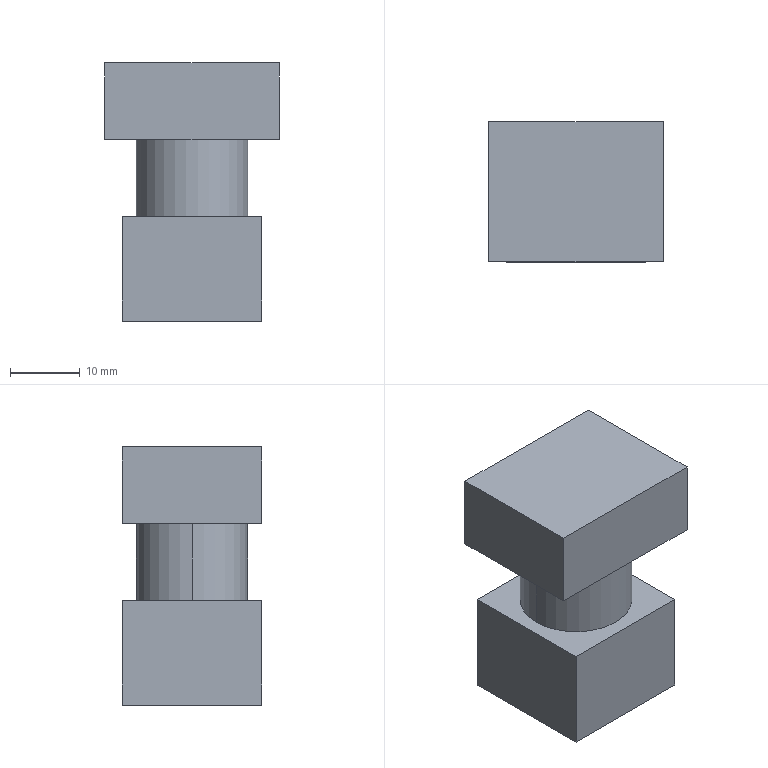Part | STEP file | Indicator light red | 1 solid | 14 faces | box 25 x 20 x 37 mm | volume 13712 mm3 | plane 12 | cylinder 2 | commonest cylinder face diameters 16 x2
STEP:
#1=CARTESIAN_POINT('',(0.,0.,0.));
#2=DIRECTION('',(0.,0.,1.));
#3=DIRECTION('',(1.,0.,0.));
#4=AXIS2_PLACEMENT_3D('',#1,#2,#3);
#5=CARTESIAN_POINT('',(8.,0.,-11.));
#6=VERTEX_POINT('',#5);
#7=CARTESIAN_POINT('',(-8.,0.,-11.));
#8=VERTEX_POINT('',#7);
#9=CARTESIAN_POINT('',(0.,0.,-11.));
#10=DIRECTION('',(0.,0.,1.));
#11=DIRECTION('',(1.,0.,0.));
#12=AXIS2_PLACEMENT_3D('',#9,#10,#11);
#13=CIRCLE('',#12,8.);
#14=CARTESIAN_POINT('',(0.,0.,-11.));
#15=DIRECTION('',(0.,0.,1.));
#16=DIRECTION('',(1.,0.,0.));
#17=AXIS2_PLACEMENT_3D('',#14,#15,#16);
#18=CYLINDRICAL_SURFACE('',#17,8.);
#19=CARTESIAN_POINT('',(0.,0.));
#20=DIRECTION('',(1.,0.));
#21=VECTOR('',#20,1.);
#22=LINE('',#19,#21);
#23=(GEOMETRIC_REPRESENTATION_CONTEXT(2)PARAMETRIC_REPRESENTATION_CONTEXT()REPRESENTATION_CONTEXT('',''));
#24=DEFINITIONAL_REPRESENTATION('',(#22),#23);
#25=PCURVE('',#18,#24);
#26=CARTESIAN_POINT('',(-10.,10.,-11.));
#27=DIRECTION('',(0.,0.,1.));
#28=DIRECTION('',(1.,0.,0.));
#29=AXIS2_PLACEMENT_3D('',#26,#27,#28);
#30=PLANE('',#29);
#31=CARTESIAN_POINT('',(10.,-10.));
#32=DIRECTION('',(1.,0.));
#33=AXIS2_PLACEMENT_2D('',#31,#32);
#34=CIRCLE('',#33,8.);
#35=(GEOMETRIC_REPRESENTATION_CONTEXT(2)PARAMETRIC_REPRESENTATION_CONTEXT()REPRESENTATION_CONTEXT('',''));
#36=DEFINITIONAL_REPRESENTATION('',(#34),#35);
#37=PCURVE('',#30,#36);
#38=SURFACE_CURVE('',#13,(#25,#37),.PCURVE_S1.);
#39=EDGE_CURVE('',#6,#8,#38,.T.);
#40=ORIENTED_EDGE('',*,*,#39,.T.);
#41=CARTESIAN_POINT('',(-8.,0.,0.));
#42=VERTEX_POINT('',#41);
#43=CARTESIAN_POINT('',(-8.,0.,-11.));
#44=DIRECTION('',(0.,0.,1.));
#45=VECTOR('',#44,1.);
#46=LINE('',#43,#45);
#47=CARTESIAN_POINT('',(3.142,0.));
#48=DIRECTION('',(0.,1.));
#49=VECTOR('',#48,1.);
#50=LINE('',#47,#49);
#51=(GEOMETRIC_REPRESENTATION_CONTEXT(2)PARAMETRIC_REPRESENTATION_CONTEXT()REPRESENTATION_CONTEXT('',''));
#52=DEFINITIONAL_REPRESENTATION('',(#50),#51);
#53=PCURVE('',#18,#52);
#54=CARTESIAN_POINT('',(0.,0.,-11.));
#55=DIRECTION('',(0.,0.,1.));
#56=DIRECTION('',(1.,0.,0.));
#57=AXIS2_PLACEMENT_3D('',#54,#55,#56);
#58=CYLINDRICAL_SURFACE('',#57,8.);
#59=CARTESIAN_POINT('',(3.142,0.));
#60=DIRECTION('',(0.,1.));
#61=VECTOR('',#60,1.);
#62=LINE('',#59,#61);
#63=(GEOMETRIC_REPRESENTATION_CONTEXT(2)PARAMETRIC_REPRESENTATION_CONTEXT()REPRESENTATION_CONTEXT('',''));
#64=DEFINITIONAL_REPRESENTATION('',(#62),#63);
#65=PCURVE('',#58,#64);
#66=SURFACE_CURVE('',#46,(#53,#65),.PCURVE_S1.);
#67=EDGE_CURVE('',#8,#42,#66,.T.);
#68=ORIENTED_EDGE('',*,*,#67,.T.);
#69=CARTESIAN_POINT('',(8.,0.,0.));
#70=VERTEX_POINT('',#69);
#71=CARTESIAN_POINT('',(0.,0.,0.));
#72=DIRECTION('',(0.,0.,-1.));
#73=DIRECTION('',(1.,0.,0.));
#74=AXIS2_PLACEMENT_3D('',#71,#72,#73);
#75=CIRCLE('',#74,8.);
#76=CARTESIAN_POINT('',(6.283,11.));
#77=DIRECTION('',(-1.,0.));
#78=VECTOR('',#77,1.);
#79=LINE('',#76,#78);
#80=(GEOMETRIC_REPRESENTATION_CONTEXT(2)PARAMETRIC_REPRESENTATION_CONTEXT()REPRESENTATION_CONTEXT('',''));
#81=DEFINITIONAL_REPRESENTATION('',(#79),#80);
#82=PCURVE('',#18,#81);
#83=CARTESIAN_POINT('',(12.5,-10.,0.));
#84=DIRECTION('',(0.,0.,1.));
#85=DIRECTION('',(1.,0.,0.));
#86=AXIS2_PLACEMENT_3D('',#83,#84,#85);
#87=PLANE('',#86);
#88=CARTESIAN_POINT('',(-4.5,10.));
#89=CARTESIAN_POINT('',(-4.5,-3.856));
#90=CARTESIAN_POINT('',(-16.5,3.072));
#91=CARTESIAN_POINT('',(-28.5,10.));
#92=CARTESIAN_POINT('',(-16.5,16.928));
#93=CARTESIAN_POINT('',(-4.5,23.856));
#94=CARTESIAN_POINT('',(-4.5,10.));
#95=(BOUNDED_CURVE()B_SPLINE_CURVE(2,(#88,#89,#90,#91,#92,#93,#94),.UNSPECIFIED.,.T.,.F.)B_SPLINE_CURVE_WITH_KNOTS((1,2,2,2,2,1),(-2.094,0.,2.094,4.189,6.283,8.378),.UNSPECIFIED.)CURVE()GEOMETRIC_REPRESENTATION_ITEM()RATIONAL_B_SPLINE_CURVE((1.,0.5,1.,0.5,1.,0.5,1.))REPRESENTATION_ITEM(''));
#96=(GEOMETRIC_REPRESENTATION_CONTEXT(2)PARAMETRIC_REPRESENTATION_CONTEXT()REPRESENTATION_CONTEXT('',''));
#97=DEFINITIONAL_REPRESENTATION('',(#95),#96);
#98=PCURVE('',#87,#97);
#99=SURFACE_CURVE('',#75,(#82,#98),.PCURVE_S1.);
#100=EDGE_CURVE('',#42,#70,#99,.T.);
#101=ORIENTED_EDGE('',*,*,#100,.T.);
#102=CARTESIAN_POINT('',(8.,0.,-11.));
#103=DIRECTION('',(0.,0.,1.));
#104=VECTOR('',#103,1.);
#105=LINE('',#102,#104);
#106=CARTESIAN_POINT('',(0.,0.));
#107=DIRECTION('',(0.,1.));
#108=VECTOR('',#107,1.);
#109=LINE('',#106,#108);
#110=(GEOMETRIC_REPRESENTATION_CONTEXT(2)PARAMETRIC_REPRESENTATION_CONTEXT()REPRESENTATION_CONTEXT('',''));
#111=DEFINITIONAL_REPRESENTATION('',(#109),#110);
#112=PCURVE('',#18,#111);
#113=CARTESIAN_POINT('',(6.283,0.));
#114=DIRECTION('',(0.,1.));
#115=VECTOR('',#114,1.);
#116=LINE('',#113,#115);
#117=(GEOMETRIC_REPRESENTATION_CONTEXT(2)PARAMETRIC_REPRESENTATION_CONTEXT()REPRESENTATION_CONTEXT('',''));
#118=DEFINITIONAL_REPRESENTATION('',(#116),#117);
#119=PCURVE('',#58,#118);
#120=SURFACE_CURVE('',#105,(#112,#119),.PCURVE_S1.);
#121=EDGE_CURVE('',#6,#70,#120,.T.);
#122=ORIENTED_EDGE('',*,*,#121,.F.);
#123=EDGE_LOOP('',(#40,#68,#101,#122));
#124=FACE_BOUND('',#123,.T.);
#125=ADVANCED_FACE('',(#124),#18,.T.);
#126=CARTESIAN_POINT('',(-12.5,10.,11.));
#127=VERTEX_POINT('',#126);
#128=CARTESIAN_POINT('',(-12.5,-10.,11.));
#129=VERTEX_POINT('',#128);
#130=CARTESIAN_POINT('',(-12.5,-10.,11.));
#131=DIRECTION('',(0.,-1.,0.));
#132=VECTOR('',#131,1.);
#133=LINE('',#130,#132);
#134=CARTESIAN_POINT('',(12.5,-10.,11.));
#135=DIRECTION('',(0.,0.,1.));
#136=DIRECTION('',(1.,0.,0.));
#137=AXIS2_PLACEMENT_3D('',#134,#135,#136);
#138=PLANE('',#137);
#139=CARTESIAN_POINT('',(-25.,0.));
#140=DIRECTION('',(0.,-1.));
#141=VECTOR('',#140,1.);
#142=LINE('',#139,#141);
#143=(GEOMETRIC_REPRESENTATION_CONTEXT(2)PARAMETRIC_REPRESENTATION_CONTEXT()REPRESENTATION_CONTEXT('',''));
#144=DEFINITIONAL_REPRESENTATION('',(#142),#143);
#145=PCURVE('',#138,#144);
#146=CARTESIAN_POINT('',(-12.5,10.,11.));
#147=DIRECTION('',(1.,0.,0.));
#148=DIRECTION('',(0.,1.,0.));
#149=AXIS2_PLACEMENT_3D('',#146,#147,#148);
#150=PLANE('',#149);
#151=CARTESIAN_POINT('',(-20.,0.));
#152=DIRECTION('',(-1.,0.));
#153=VECTOR('',#152,1.);
#154=LINE('',#151,#153);
#155=(GEOMETRIC_REPRESENTATION_CONTEXT(2)PARAMETRIC_REPRESENTATION_CONTEXT()REPRESENTATION_CONTEXT('',''));
#156=DEFINITIONAL_REPRESENTATION('',(#154),#155);
#157=PCURVE('',#150,#156);
#158=SURFACE_CURVE('',#133,(#145,#157),.PCURVE_S1.);
#159=EDGE_CURVE('',#127,#129,#158,.T.);
#160=ORIENTED_EDGE('',*,*,#159,.T.);
#161=CARTESIAN_POINT('',(12.5,-10.,11.));
#162=VERTEX_POINT('',#161);
#163=CARTESIAN_POINT('',(12.5,-10.,11.));
#164=DIRECTION('',(1.,0.,0.));
#165=VECTOR('',#164,1.);
#166=LINE('',#163,#165);
#167=CARTESIAN_POINT('',(0.,0.));
#168=DIRECTION('',(1.,0.));
#169=VECTOR('',#168,1.);
#170=LINE('',#167,#169);
#171=(GEOMETRIC_REPRESENTATION_CONTEXT(2)PARAMETRIC_REPRESENTATION_CONTEXT()REPRESENTATION_CONTEXT('',''));
#172=DEFINITIONAL_REPRESENTATION('',(#170),#171);
#173=PCURVE('',#138,#172);
#174=CARTESIAN_POINT('',(-12.5,-10.,11.));
#175=DIRECTION('',(0.,1.,0.));
#176=DIRECTION('',(0.,0.,1.));
#177=AXIS2_PLACEMENT_3D('',#174,#175,#176);
#178=PLANE('',#177);
#179=CARTESIAN_POINT('',(0.,25.));
#180=DIRECTION('',(0.,1.));
#181=VECTOR('',#180,1.);
#182=LINE('',#179,#181);
#183=(GEOMETRIC_REPRESENTATION_CONTEXT(2)PARAMETRIC_REPRESENTATION_CONTEXT()REPRESENTATION_CONTEXT('',''));
#184=DEFINITIONAL_REPRESENTATION('',(#182),#183);
#185=PCURVE('',#178,#184);
#186=SURFACE_CURVE('',#166,(#173,#185),.PCURVE_S1.);
#187=EDGE_CURVE('',#129,#162,#186,.T.);
#188=ORIENTED_EDGE('',*,*,#187,.T.);
#189=CARTESIAN_POINT('',(12.5,10.,11.));
#190=VERTEX_POINT('',#189);
#191=CARTESIAN_POINT('',(12.5,-10.,11.));
#192=DIRECTION('',(0.,1.,0.));
#193=VECTOR('',#192,1.);
#194=LINE('',#191,#193);
#195=CARTESIAN_POINT('',(0.,0.));
#196=DIRECTION('',(0.,1.));
#197=VECTOR('',#196,1.);
#198=LINE('',#195,#197);
#199=(GEOMETRIC_REPRESENTATION_CONTEXT(2)PARAMETRIC_REPRESENTATION_CONTEXT()REPRESENTATION_CONTEXT('',''));
#200=DEFINITIONAL_REPRESENTATION('',(#198),#199);
#201=PCURVE('',#138,#200);
#202=CARTESIAN_POINT('',(12.5,10.,11.));
#203=DIRECTION('',(-1.,0.,0.));
#204=DIRECTION('',(0.,-1.,0.));
#205=AXIS2_PLACEMENT_3D('',#202,#203,#204);
#206=PLANE('',#205);
#207=CARTESIAN_POINT('',(20.,0.));
#208=DIRECTION('',(-1.,0.));
#209=VECTOR('',#208,1.);
#210=LINE('',#207,#209);
#211=(GEOMETRIC_REPRESENTATION_CONTEXT(2)PARAMETRIC_REPRESENTATION_CONTEXT()REPRESENTATION_CONTEXT('',''));
#212=DEFINITIONAL_REPRESENTATION('',(#210),#211);
#213=PCURVE('',#206,#212);
#214=SURFACE_CURVE('',#194,(#201,#213),.PCURVE_S1.);
#215=EDGE_CURVE('',#162,#190,#214,.T.);
#216=ORIENTED_EDGE('',*,*,#215,.T.);
#217=CARTESIAN_POINT('',(12.5,10.,11.));
#218=DIRECTION('',(-1.,0.,0.));
#219=VECTOR('',#218,1.);
#220=LINE('',#217,#219);
#221=CARTESIAN_POINT('',(0.,20.));
#222=DIRECTION('',(-1.,0.));
#223=VECTOR('',#222,1.);
#224=LINE('',#221,#223);
#225=(GEOMETRIC_REPRESENTATION_CONTEXT(2)PARAMETRIC_REPRESENTATION_CONTEXT()REPRESENTATION_CONTEXT('',''));
#226=DEFINITIONAL_REPRESENTATION('',(#224),#225);
#227=PCURVE('',#138,#226);
#228=CARTESIAN_POINT('',(-12.5,10.,11.));
#229=DIRECTION('',(0.,-1.,0.));
#230=DIRECTION('',(0.,0.,-1.));
#231=AXIS2_PLACEMENT_3D('',#228,#229,#230);
#232=PLANE('',#231);
#233=CARTESIAN_POINT('',(0.,25.));
#234=DIRECTION('',(0.,-1.));
#235=VECTOR('',#234,1.);
#236=LINE('',#233,#235);
#237=(GEOMETRIC_REPRESENTATION_CONTEXT(2)PARAMETRIC_REPRESENTATION_CONTEXT()REPRESENTATION_CONTEXT('',''));
#238=DEFINITIONAL_REPRESENTATION('',(#236),#237);
#239=PCURVE('',#232,#238);
#240=SURFACE_CURVE('',#220,(#227,#239),.PCURVE_S1.);
#241=EDGE_CURVE('',#190,#127,#240,.T.);
#242=ORIENTED_EDGE('',*,*,#241,.T.);
#243=EDGE_LOOP('',(#160,#188,#216,#242));
#244=FACE_BOUND('',#243,.T.);
#245=ADVANCED_FACE('',(#244),#138,.T.);
#246=CARTESIAN_POINT('',(12.5,-10.,0.));
#247=VERTEX_POINT('',#246);
#248=CARTESIAN_POINT('',(12.5,-10.,11.));
#249=DIRECTION('',(0.,0.,-1.));
#250=VECTOR('',#249,1.);
#251=LINE('',#248,#250);
#252=CARTESIAN_POINT('',(0.,25.));
#253=DIRECTION('',(-1.,0.));
#254=VECTOR('',#253,1.);
#255=LINE('',#252,#254);
#256=(GEOMETRIC_REPRESENTATION_CONTEXT(2)PARAMETRIC_REPRESENTATION_CONTEXT()REPRESENTATION_CONTEXT('',''));
#257=DEFINITIONAL_REPRESENTATION('',(#255),#256);
#258=PCURVE('',#178,#257);
#259=CARTESIAN_POINT('',(20.,0.));
#260=DIRECTION('',(0.,-1.));
#261=VECTOR('',#260,1.);
#262=LINE('',#259,#261);
#263=(GEOMETRIC_REPRESENTATION_CONTEXT(2)PARAMETRIC_REPRESENTATION_CONTEXT()REPRESENTATION_CONTEXT('',''));
#264=DEFINITIONAL_REPRESENTATION('',(#262),#263);
#265=PCURVE('',#206,#264);
#266=SURFACE_CURVE('',#251,(#258,#265),.PCURVE_S1.);
#267=EDGE_CURVE('',#162,#247,#266,.T.);
#268=ORIENTED_EDGE('',*,*,#267,.F.);
#269=ORIENTED_EDGE('',*,*,#187,.F.);
#270=CARTESIAN_POINT('',(-12.5,-10.,0.));
#271=VERTEX_POINT('',#270);
#272=CARTESIAN_POINT('',(-12.5,-10.,11.));
#273=DIRECTION('',(0.,0.,1.));
#274=VECTOR('',#273,1.);
#275=LINE('',#272,#274);
#276=CARTESIAN_POINT('',(0.,0.));
#277=DIRECTION('',(1.,0.));
#278=VECTOR('',#277,1.);
#279=LINE('',#276,#278);
#280=(GEOMETRIC_REPRESENTATION_CONTEXT(2)PARAMETRIC_REPRESENTATION_CONTEXT()REPRESENTATION_CONTEXT('',''));
#281=DEFINITIONAL_REPRESENTATION('',(#279),#280);
#282=PCURVE('',#178,#281);
#283=CARTESIAN_POINT('',(-20.,0.));
#284=DIRECTION('',(0.,1.));
#285=VECTOR('',#284,1.);
#286=LINE('',#283,#285);
#287=(GEOMETRIC_REPRESENTATION_CONTEXT(2)PARAMETRIC_REPRESENTATION_CONTEXT()REPRESENTATION_CONTEXT('',''));
#288=DEFINITIONAL_REPRESENTATION('',(#286),#287);
#289=PCURVE('',#150,#288);
#290=SURFACE_CURVE('',#275,(#282,#289),.PCURVE_S1.);
#291=EDGE_CURVE('',#271,#129,#290,.T.);
#292=ORIENTED_EDGE('',*,*,#291,.F.);
#293=CARTESIAN_POINT('',(-12.5,-10.,0.));
#294=DIRECTION('',(-1.,0.,0.));
#295=VECTOR('',#294,1.);
#296=LINE('',#293,#295);
#297=CARTESIAN_POINT('',(-11.,0.));
#298=DIRECTION('',(0.,-1.));
#299=VECTOR('',#298,1.);
#300=LINE('',#297,#299);
#301=(GEOMETRIC_REPRESENTATION_CONTEXT(2)PARAMETRIC_REPRESENTATION_CONTEXT()REPRESENTATION_CONTEXT('',''));
#302=DEFINITIONAL_REPRESENTATION('',(#300),#301);
#303=PCURVE('',#178,#302);
#304=CARTESIAN_POINT('',(-25.,0.));
#305=DIRECTION('',(-1.,0.));
#306=VECTOR('',#305,1.);
#307=LINE('',#304,#306);
#308=(GEOMETRIC_REPRESENTATION_CONTEXT(2)PARAMETRIC_REPRESENTATION_CONTEXT()REPRESENTATION_CONTEXT('',''));
#309=DEFINITIONAL_REPRESENTATION('',(#307),#308);
#310=PCURVE('',#87,#309);
#311=SURFACE_CURVE('',#296,(#303,#310),.PCURVE_S1.);
#312=EDGE_CURVE('',#247,#271,#311,.T.);
#313=ORIENTED_EDGE('',*,*,#312,.F.);
#314=EDGE_LOOP('',(#268,#269,#292,#313));
#315=FACE_BOUND('',#314,.T.);
#316=ADVANCED_FACE('',(#315),#178,.F.);
#317=ORIENTED_EDGE('',*,*,#291,.T.);
#318=ORIENTED_EDGE('',*,*,#159,.F.);
#319=CARTESIAN_POINT('',(-12.5,10.,0.));
#320=VERTEX_POINT('',#319);
#321=CARTESIAN_POINT('',(-12.5,10.,11.));
#322=DIRECTION('',(0.,0.,1.));
#323=VECTOR('',#322,1.);
#324=LINE('',#321,#323);
#325=CARTESIAN_POINT('',(0.,0.));
#326=DIRECTION('',(0.,1.));
#327=VECTOR('',#326,1.);
#328=LINE('',#325,#327);
#329=(GEOMETRIC_REPRESENTATION_CONTEXT(2)PARAMETRIC_REPRESENTATION_CONTEXT()REPRESENTATION_CONTEXT('',''));
#330=DEFINITIONAL_REPRESENTATION('',(#328),#329);
#331=PCURVE('',#150,#330);
#332=CARTESIAN_POINT('',(0.,0.));
#333=DIRECTION('',(-1.,0.));
#334=VECTOR('',#333,1.);
#335=LINE('',#332,#334);
#336=(GEOMETRIC_REPRESENTATION_CONTEXT(2)PARAMETRIC_REPRESENTATION_CONTEXT()REPRESENTATION_CONTEXT('',''));
#337=DEFINITIONAL_REPRESENTATION('',(#335),#336);
#338=PCURVE('',#232,#337);
#339=SURFACE_CURVE('',#324,(#331,#338),.PCURVE_S1.);
#340=EDGE_CURVE('',#320,#127,#339,.T.);
#341=ORIENTED_EDGE('',*,*,#340,.F.);
#342=CARTESIAN_POINT('',(-12.5,10.,0.));
#343=DIRECTION('',(0.,1.,0.));
#344=VECTOR('',#343,1.);
#345=LINE('',#342,#344);
#346=CARTESIAN_POINT('',(0.,-11.));
#347=DIRECTION('',(1.,0.));
#348=VECTOR('',#347,1.);
#349=LINE('',#346,#348);
#350=(GEOMETRIC_REPRESENTATION_CONTEXT(2)PARAMETRIC_REPRESENTATION_CONTEXT()REPRESENTATION_CONTEXT('',''));
#351=DEFINITIONAL_REPRESENTATION('',(#349),#350);
#352=PCURVE('',#150,#351);
#353=CARTESIAN_POINT('',(-25.,20.));
#354=DIRECTION('',(0.,1.));
#355=VECTOR('',#354,1.);
#356=LINE('',#353,#355);
#357=(GEOMETRIC_REPRESENTATION_CONTEXT(2)PARAMETRIC_REPRESENTATION_CONTEXT()REPRESENTATION_CONTEXT('',''));
#358=DEFINITIONAL_REPRESENTATION('',(#356),#357);
#359=PCURVE('',#87,#358);
#360=SURFACE_CURVE('',#345,(#352,#359),.PCURVE_S1.);
#361=EDGE_CURVE('',#271,#320,#360,.T.);
#362=ORIENTED_EDGE('',*,*,#361,.F.);
#363=EDGE_LOOP('',(#317,#318,#341,#362));
#364=FACE_BOUND('',#363,.T.);
#365=ADVANCED_FACE('',(#364),#150,.F.);
#366=ORIENTED_EDGE('',*,*,#340,.T.);
#367=ORIENTED_EDGE('',*,*,#241,.F.);
#368=CARTESIAN_POINT('',(12.5,10.,0.));
#369=VERTEX_POINT('',#368);
#370=CARTESIAN_POINT('',(12.5,10.,11.));
#371=DIRECTION('',(0.,0.,1.));
#372=VECTOR('',#371,1.);
#373=LINE('',#370,#372);
#374=CARTESIAN_POINT('',(0.,25.));
#375=DIRECTION('',(-1.,0.));
#376=VECTOR('',#375,1.);
#377=LINE('',#374,#376);
#378=(GEOMETRIC_REPRESENTATION_CONTEXT(2)PARAMETRIC_REPRESENTATION_CONTEXT()REPRESENTATION_CONTEXT('',''));
#379=DEFINITIONAL_REPRESENTATION('',(#377),#378);
#380=PCURVE('',#232,#379);
#381=CARTESIAN_POINT('',(0.,0.));
#382=DIRECTION('',(0.,1.));
#383=VECTOR('',#382,1.);
#384=LINE('',#381,#383);
#385=(GEOMETRIC_REPRESENTATION_CONTEXT(2)PARAMETRIC_REPRESENTATION_CONTEXT()REPRESENTATION_CONTEXT('',''));
#386=DEFINITIONAL_REPRESENTATION('',(#384),#385);
#387=PCURVE('',#206,#386);
#388=SURFACE_CURVE('',#373,(#380,#387),.PCURVE_S1.);
#389=EDGE_CURVE('',#369,#190,#388,.T.);
#390=ORIENTED_EDGE('',*,*,#389,.F.);
#391=CARTESIAN_POINT('',(-12.5,10.,0.));
#392=DIRECTION('',(1.,0.,0.));
#393=VECTOR('',#392,1.);
#394=LINE('',#391,#393);
#395=CARTESIAN_POINT('',(11.,0.));
#396=DIRECTION('',(0.,1.));
#397=VECTOR('',#396,1.);
#398=LINE('',#395,#397);
#399=(GEOMETRIC_REPRESENTATION_CONTEXT(2)PARAMETRIC_REPRESENTATION_CONTEXT()REPRESENTATION_CONTEXT('',''));
#400=DEFINITIONAL_REPRESENTATION('',(#398),#399);
#401=PCURVE('',#232,#400);
#402=CARTESIAN_POINT('',(-25.,20.));
#403=DIRECTION('',(1.,0.));
#404=VECTOR('',#403,1.);
#405=LINE('',#402,#404);
#406=(GEOMETRIC_REPRESENTATION_CONTEXT(2)PARAMETRIC_REPRESENTATION_CONTEXT()REPRESENTATION_CONTEXT('',''));
#407=DEFINITIONAL_REPRESENTATION('',(#405),#406);
#408=PCURVE('',#87,#407);
#409=SURFACE_CURVE('',#394,(#401,#408),.PCURVE_S1.);
#410=EDGE_CURVE('',#320,#369,#409,.T.);
#411=ORIENTED_EDGE('',*,*,#410,.F.);
#412=EDGE_LOOP('',(#366,#367,#390,#411));
#413=FACE_BOUND('',#412,.T.);
#414=ADVANCED_FACE('',(#413),#232,.F.);
#415=ORIENTED_EDGE('',*,*,#389,.T.);
#416=ORIENTED_EDGE('',*,*,#215,.F.);
#417=ORIENTED_EDGE('',*,*,#267,.T.);
#418=CARTESIAN_POINT('',(12.5,10.,0.));
#419=DIRECTION('',(0.,-1.,0.));
#420=VECTOR('',#419,1.);
#421=LINE('',#418,#420);
#422=CARTESIAN_POINT('',(0.,-11.));
#423=DIRECTION('',(1.,0.));
#424=VECTOR('',#423,1.);
#425=LINE('',#422,#424);
#426=(GEOMETRIC_REPRESENTATION_CONTEXT(2)PARAMETRIC_REPRESENTATION_CONTEXT()REPRESENTATION_CONTEXT('',''));
#427=DEFINITIONAL_REPRESENTATION('',(#425),#426);
#428=PCURVE('',#206,#427);
#429=CARTESIAN_POINT('',(0.,20.));
#430=DIRECTION('',(0.,-1.));
#431=VECTOR('',#430,1.);
#432=LINE('',#429,#431);
#433=(GEOMETRIC_REPRESENTATION_CONTEXT(2)PARAMETRIC_REPRESENTATION_CONTEXT()REPRESENTATION_CONTEXT('',''));
#434=DEFINITIONAL_REPRESENTATION('',(#432),#433);
#435=PCURVE('',#87,#434);
#436=SURFACE_CURVE('',#421,(#428,#435),.PCURVE_S1.);
#437=EDGE_CURVE('',#369,#247,#436,.T.);
#438=ORIENTED_EDGE('',*,*,#437,.F.);
#439=EDGE_LOOP('',(#415,#416,#417,#438));
#440=FACE_BOUND('',#439,.T.);
#441=ADVANCED_FACE('',(#440),#206,.F.);
#442=CARTESIAN_POINT('',(0.,0.,0.));
#443=DIRECTION('',(0.,0.,-1.));
#444=DIRECTION('',(1.,0.,0.));
#445=AXIS2_PLACEMENT_3D('',#442,#443,#444);
#446=CIRCLE('',#445,8.);
#447=CARTESIAN_POINT('',(-4.5,10.));
#448=CARTESIAN_POINT('',(-4.5,-3.856));
#449=CARTESIAN_POINT('',(-16.5,3.072));
#450=CARTESIAN_POINT('',(-28.5,10.));
#451=CARTESIAN_POINT('',(-16.5,16.928));
#452=CARTESIAN_POINT('',(-4.5,23.856));
#453=CARTESIAN_POINT('',(-4.5,10.));
#454=(BOUNDED_CURVE()B_SPLINE_CURVE(2,(#447,#448,#449,#450,#451,#452,#453),.UNSPECIFIED.,.T.,.F.)B_SPLINE_CURVE_WITH_KNOTS((1,2,2,2,2,1),(-2.094,0.,2.094,4.189,6.283,8.378),.UNSPECIFIED.)CURVE()GEOMETRIC_REPRESENTATION_ITEM()RATIONAL_B_SPLINE_CURVE((1.,0.5,1.,0.5,1.,0.5,1.))REPRESENTATION_ITEM(''));
#455=(GEOMETRIC_REPRESENTATION_CONTEXT(2)PARAMETRIC_REPRESENTATION_CONTEXT()REPRESENTATION_CONTEXT('',''));
#456=DEFINITIONAL_REPRESENTATION('',(#454),#455);
#457=PCURVE('',#87,#456);
#458=CARTESIAN_POINT('',(6.283,11.));
#459=DIRECTION('',(-1.,0.));
#460=VECTOR('',#459,1.);
#461=LINE('',#458,#460);
#462=(GEOMETRIC_REPRESENTATION_CONTEXT(2)PARAMETRIC_REPRESENTATION_CONTEXT()REPRESENTATION_CONTEXT('',''));
#463=DEFINITIONAL_REPRESENTATION('',(#461),#462);
#464=PCURVE('',#58,#463);
#465=SURFACE_CURVE('',#446,(#457,#464),.PCURVE_S1.);
#466=EDGE_CURVE('',#70,#42,#465,.T.);
#467=ORIENTED_EDGE('',*,*,#466,.F.);
#468=ORIENTED_EDGE('',*,*,#100,.F.);
#469=EDGE_LOOP('',(#467,#468));
#470=FACE_BOUND('',#469,.T.);
#471=ORIENTED_EDGE('',*,*,#312,.T.);
#472=ORIENTED_EDGE('',*,*,#361,.T.);
#473=ORIENTED_EDGE('',*,*,#410,.T.);
#474=ORIENTED_EDGE('',*,*,#437,.T.);
#475=EDGE_LOOP('',(#471,#472,#473,#474));
#476=FACE_BOUND('',#475,.T.);
#477=ADVANCED_FACE('',(#470,#476),#87,.F.);
#478=ORIENTED_EDGE('',*,*,#67,.F.);
#479=CARTESIAN_POINT('',(0.,0.,-11.));
#480=DIRECTION('',(0.,0.,1.));
#481=DIRECTION('',(1.,0.,0.));
#482=AXIS2_PLACEMENT_3D('',#479,#480,#481);
#483=CIRCLE('',#482,8.);
#484=CARTESIAN_POINT('',(0.,0.));
#485=DIRECTION('',(1.,0.));
#486=VECTOR('',#485,1.);
#487=LINE('',#484,#486);
#488=(GEOMETRIC_REPRESENTATION_CONTEXT(2)PARAMETRIC_REPRESENTATION_CONTEXT()REPRESENTATION_CONTEXT('',''));
#489=DEFINITIONAL_REPRESENTATION('',(#487),#488);
#490=PCURVE('',#58,#489);
#491=CARTESIAN_POINT('',(10.,-10.));
#492=DIRECTION('',(1.,0.));
#493=AXIS2_PLACEMENT_2D('',#491,#492);
#494=CIRCLE('',#493,8.);
#495=(GEOMETRIC_REPRESENTATION_CONTEXT(2)PARAMETRIC_REPRESENTATION_CONTEXT()REPRESENTATION_CONTEXT('',''));
#496=DEFINITIONAL_REPRESENTATION('',(#494),#495);
#497=PCURVE('',#30,#496);
#498=SURFACE_CURVE('',#483,(#490,#497),.PCURVE_S1.);
#499=EDGE_CURVE('',#8,#6,#498,.T.);
#500=ORIENTED_EDGE('',*,*,#499,.T.);
#501=ORIENTED_EDGE('',*,*,#121,.T.);
#502=ORIENTED_EDGE('',*,*,#466,.T.);
#503=EDGE_LOOP('',(#478,#500,#501,#502));
#504=FACE_BOUND('',#503,.T.);
#505=ADVANCED_FACE('',(#504),#58,.T.);
#506=ORIENTED_EDGE('',*,*,#39,.F.);
#507=ORIENTED_EDGE('',*,*,#499,.F.);
#508=EDGE_LOOP('',(#506,#507));
#509=FACE_BOUND('',#508,.T.);
#510=CARTESIAN_POINT('',(10.,-10.,-11.));
#511=VERTEX_POINT('',#510);
#512=CARTESIAN_POINT('',(10.,10.,-11.));
#513=VERTEX_POINT('',#512);
#514=CARTESIAN_POINT('',(10.,10.,-11.));
#515=DIRECTION('',(0.,1.,0.));
#516=VECTOR('',#515,1.);
#517=LINE('',#514,#516);
#518=CARTESIAN_POINT('',(20.,0.));
#519=DIRECTION('',(0.,1.));
#520=VECTOR('',#519,1.);
#521=LINE('',#518,#520);
#522=(GEOMETRIC_REPRESENTATION_CONTEXT(2)PARAMETRIC_REPRESENTATION_CONTEXT()REPRESENTATION_CONTEXT('',''));
#523=DEFINITIONAL_REPRESENTATION('',(#521),#522);
#524=PCURVE('',#30,#523);
#525=CARTESIAN_POINT('',(10.,-10.,-26.));
#526=DIRECTION('',(-1.,0.,0.));
#527=DIRECTION('',(0.,0.,1.));
#528=AXIS2_PLACEMENT_3D('',#525,#526,#527);
#529=PLANE('',#528);
#530=CARTESIAN_POINT('',(15.,20.));
#531=DIRECTION('',(0.,1.));
#532=VECTOR('',#531,1.);
#533=LINE('',#530,#532);
#534=(GEOMETRIC_REPRESENTATION_CONTEXT(2)PARAMETRIC_REPRESENTATION_CONTEXT()REPRESENTATION_CONTEXT('',''));
#535=DEFINITIONAL_REPRESENTATION('',(#533),#534);
#536=PCURVE('',#529,#535);
#537=SURFACE_CURVE('',#517,(#524,#536),.PCURVE_S1.);
#538=EDGE_CURVE('',#511,#513,#537,.T.);
#539=ORIENTED_EDGE('',*,*,#538,.T.);
#540=CARTESIAN_POINT('',(-10.,10.,-11.));
#541=VERTEX_POINT('',#540);
#542=CARTESIAN_POINT('',(-10.,10.,-11.));
#543=DIRECTION('',(-1.,0.,0.));
#544=VECTOR('',#543,1.);
#545=LINE('',#542,#544);
#546=CARTESIAN_POINT('',(0.,0.));
#547=DIRECTION('',(-1.,0.));
#548=VECTOR('',#547,1.);
#549=LINE('',#546,#548);
#550=(GEOMETRIC_REPRESENTATION_CONTEXT(2)PARAMETRIC_REPRESENTATION_CONTEXT()REPRESENTATION_CONTEXT('',''));
#551=DEFINITIONAL_REPRESENTATION('',(#549),#550);
#552=PCURVE('',#30,#551);
#553=CARTESIAN_POINT('',(10.,10.,-26.));
#554=DIRECTION('',(0.,-1.,0.));
#555=DIRECTION('',(0.,0.,-1.));
#556=AXIS2_PLACEMENT_3D('',#553,#554,#555);
#557=PLANE('',#556);
#558=CARTESIAN_POINT('',(-15.,-20.));
#559=DIRECTION('',(0.,-1.));
#560=VECTOR('',#559,1.);
#561=LINE('',#558,#560);
#562=(GEOMETRIC_REPRESENTATION_CONTEXT(2)PARAMETRIC_REPRESENTATION_CONTEXT()REPRESENTATION_CONTEXT('',''));
#563=DEFINITIONAL_REPRESENTATION('',(#561),#562);
#564=PCURVE('',#557,#563);
#565=SURFACE_CURVE('',#545,(#552,#564),.PCURVE_S1.);
#566=EDGE_CURVE('',#513,#541,#565,.T.);
#567=ORIENTED_EDGE('',*,*,#566,.T.);
#568=CARTESIAN_POINT('',(-10.,-10.,-11.));
#569=VERTEX_POINT('',#568);
#570=CARTESIAN_POINT('',(-10.,10.,-11.));
#571=DIRECTION('',(0.,-1.,0.));
#572=VECTOR('',#571,1.);
#573=LINE('',#570,#572);
#574=CARTESIAN_POINT('',(0.,0.));
#575=DIRECTION('',(0.,-1.));
#576=VECTOR('',#575,1.);
#577=LINE('',#574,#576);
#578=(GEOMETRIC_REPRESENTATION_CONTEXT(2)PARAMETRIC_REPRESENTATION_CONTEXT()REPRESENTATION_CONTEXT('',''));
#579=DEFINITIONAL_REPRESENTATION('',(#577),#578);
#580=PCURVE('',#30,#579);
#581=CARTESIAN_POINT('',(-10.,-10.,-26.));
#582=DIRECTION('',(1.,0.,0.));
#583=DIRECTION('',(0.,0.,-1.));
#584=AXIS2_PLACEMENT_3D('',#581,#582,#583);
#585=PLANE('',#584);
#586=CARTESIAN_POINT('',(-15.,20.));
#587=DIRECTION('',(0.,-1.));
#588=VECTOR('',#587,1.);
#589=LINE('',#586,#588);
#590=(GEOMETRIC_REPRESENTATION_CONTEXT(2)PARAMETRIC_REPRESENTATION_CONTEXT()REPRESENTATION_CONTEXT('',''));
#591=DEFINITIONAL_REPRESENTATION('',(#589),#590);
#592=PCURVE('',#585,#591);
#593=SURFACE_CURVE('',#573,(#580,#592),.PCURVE_S1.);
#594=EDGE_CURVE('',#541,#569,#593,.T.);
#595=ORIENTED_EDGE('',*,*,#594,.T.);
#596=CARTESIAN_POINT('',(-10.,-10.,-11.));
#597=DIRECTION('',(1.,0.,0.));
#598=VECTOR('',#597,1.);
#599=LINE('',#596,#598);
#600=CARTESIAN_POINT('',(0.,-20.));
#601=DIRECTION('',(1.,0.));
#602=VECTOR('',#601,1.);
#603=LINE('',#600,#602);
#604=(GEOMETRIC_REPRESENTATION_CONTEXT(2)PARAMETRIC_REPRESENTATION_CONTEXT()REPRESENTATION_CONTEXT('',''));
#605=DEFINITIONAL_REPRESENTATION('',(#603),#604);
#606=PCURVE('',#30,#605);
#607=CARTESIAN_POINT('',(10.,-10.,-26.));
#608=DIRECTION('',(0.,1.,0.));
#609=DIRECTION('',(0.,0.,1.));
#610=AXIS2_PLACEMENT_3D('',#607,#608,#609);
#611=PLANE('',#610);
#612=CARTESIAN_POINT('',(15.,-20.));
#613=DIRECTION('',(0.,1.));
#614=VECTOR('',#613,1.);
#615=LINE('',#612,#614);
#616=(GEOMETRIC_REPRESENTATION_CONTEXT(2)PARAMETRIC_REPRESENTATION_CONTEXT()REPRESENTATION_CONTEXT('',''));
#617=DEFINITIONAL_REPRESENTATION('',(#615),#616);
#618=PCURVE('',#611,#617);
#619=SURFACE_CURVE('',#599,(#606,#618),.PCURVE_S1.);
#620=EDGE_CURVE('',#569,#511,#619,.T.);
#621=ORIENTED_EDGE('',*,*,#620,.T.);
#622=EDGE_LOOP('',(#539,#567,#595,#621));
#623=FACE_BOUND('',#622,.T.);
#624=ADVANCED_FACE('',(#509,#623),#30,.T.);
#625=CARTESIAN_POINT('',(10.,10.,-26.));
#626=VERTEX_POINT('',#625);
#627=CARTESIAN_POINT('',(10.,10.,-26.));
#628=DIRECTION('',(0.,0.,1.));
#629=VECTOR('',#628,1.);
#630=LINE('',#627,#629);
#631=CARTESIAN_POINT('',(0.,0.));
#632=DIRECTION('',(-1.,0.));
#633=VECTOR('',#632,1.);
#634=LINE('',#631,#633);
#635=(GEOMETRIC_REPRESENTATION_CONTEXT(2)PARAMETRIC_REPRESENTATION_CONTEXT()REPRESENTATION_CONTEXT('',''));
#636=DEFINITIONAL_REPRESENTATION('',(#634),#635);
#637=PCURVE('',#557,#636);
#638=CARTESIAN_POINT('',(0.,20.));
#639=DIRECTION('',(1.,0.));
#640=VECTOR('',#639,1.);
#641=LINE('',#638,#640);
#642=(GEOMETRIC_REPRESENTATION_CONTEXT(2)PARAMETRIC_REPRESENTATION_CONTEXT()REPRESENTATION_CONTEXT('',''));
#643=DEFINITIONAL_REPRESENTATION('',(#641),#642);
#644=PCURVE('',#529,#643);
#645=SURFACE_CURVE('',#630,(#637,#644),.PCURVE_S1.);
#646=EDGE_CURVE('',#626,#513,#645,.T.);
#647=ORIENTED_EDGE('',*,*,#646,.F.);
#648=CARTESIAN_POINT('',(-10.,10.,-26.));
#649=VERTEX_POINT('',#648);
#650=CARTESIAN_POINT('',(10.,10.,-26.));
#651=DIRECTION('',(1.,0.,0.));
#652=VECTOR('',#651,1.);
#653=LINE('',#650,#652);
#654=CARTESIAN_POINT('',(0.,0.));
#655=DIRECTION('',(0.,1.));
#656=VECTOR('',#655,1.);
#657=LINE('',#654,#656);
#658=(GEOMETRIC_REPRESENTATION_CONTEXT(2)PARAMETRIC_REPRESENTATION_CONTEXT()REPRESENTATION_CONTEXT('',''));
#659=DEFINITIONAL_REPRESENTATION('',(#657),#658);
#660=PCURVE('',#557,#659);
#661=CARTESIAN_POINT('',(-10.,10.,-26.));
#662=DIRECTION('',(0.,0.,1.));
#663=DIRECTION('',(1.,0.,0.));
#664=AXIS2_PLACEMENT_3D('',#661,#662,#663);
#665=PLANE('',#664);
#666=CARTESIAN_POINT('',(20.,0.));
#667=DIRECTION('',(1.,0.));
#668=VECTOR('',#667,1.);
#669=LINE('',#666,#668);
#670=(GEOMETRIC_REPRESENTATION_CONTEXT(2)PARAMETRIC_REPRESENTATION_CONTEXT()REPRESENTATION_CONTEXT('',''));
#671=DEFINITIONAL_REPRESENTATION('',(#669),#670);
#672=PCURVE('',#665,#671);
#673=SURFACE_CURVE('',#653,(#660,#672),.PCURVE_S1.);
#674=EDGE_CURVE('',#649,#626,#673,.T.);
#675=ORIENTED_EDGE('',*,*,#674,.F.);
#676=CARTESIAN_POINT('',(-10.,10.,-26.));
#677=DIRECTION('',(0.,0.,-1.));
#678=VECTOR('',#677,1.);
#679=LINE('',#676,#678);
#680=CARTESIAN_POINT('',(0.,-20.));
#681=DIRECTION('',(1.,0.));
#682=VECTOR('',#681,1.);
#683=LINE('',#680,#682);
#684=(GEOMETRIC_REPRESENTATION_CONTEXT(2)PARAMETRIC_REPRESENTATION_CONTEXT()REPRESENTATION_CONTEXT('',''));
#685=DEFINITIONAL_REPRESENTATION('',(#683),#684);
#686=PCURVE('',#557,#685);
#687=CARTESIAN_POINT('',(0.,20.));
#688=DIRECTION('',(1.,0.));
#689=VECTOR('',#688,1.);
#690=LINE('',#687,#689);
#691=(GEOMETRIC_REPRESENTATION_CONTEXT(2)PARAMETRIC_REPRESENTATION_CONTEXT()REPRESENTATION_CONTEXT('',''));
#692=DEFINITIONAL_REPRESENTATION('',(#690),#691);
#693=PCURVE('',#585,#692);
#694=SURFACE_CURVE('',#679,(#686,#693),.PCURVE_S1.);
#695=EDGE_CURVE('',#541,#649,#694,.T.);
#696=ORIENTED_EDGE('',*,*,#695,.F.);
#697=ORIENTED_EDGE('',*,*,#566,.F.);
#698=EDGE_LOOP('',(#647,#675,#696,#697));
#699=FACE_BOUND('',#698,.T.);
#700=ADVANCED_FACE('',(#699),#557,.F.);
#701=CARTESIAN_POINT('',(10.,-10.,-26.));
#702=VERTEX_POINT('',#701);
#703=CARTESIAN_POINT('',(10.,-10.,-26.));
#704=DIRECTION('',(0.,0.,1.));
#705=VECTOR('',#704,1.);
#706=LINE('',#703,#705);
#707=CARTESIAN_POINT('',(0.,0.));
#708=DIRECTION('',(1.,0.));
#709=VECTOR('',#708,1.);
#710=LINE('',#707,#709);
#711=(GEOMETRIC_REPRESENTATION_CONTEXT(2)PARAMETRIC_REPRESENTATION_CONTEXT()REPRESENTATION_CONTEXT('',''));
#712=DEFINITIONAL_REPRESENTATION('',(#710),#711);
#713=PCURVE('',#529,#712);
#714=CARTESIAN_POINT('',(0.,0.));
#715=DIRECTION('',(1.,0.));
#716=VECTOR('',#715,1.);
#717=LINE('',#714,#716);
#718=(GEOMETRIC_REPRESENTATION_CONTEXT(2)PARAMETRIC_REPRESENTATION_CONTEXT()REPRESENTATION_CONTEXT('',''));
#719=DEFINITIONAL_REPRESENTATION('',(#717),#718);
#720=PCURVE('',#611,#719);
#721=SURFACE_CURVE('',#706,(#713,#720),.PCURVE_S1.);
#722=EDGE_CURVE('',#702,#511,#721,.T.);
#723=ORIENTED_EDGE('',*,*,#722,.F.);
#724=CARTESIAN_POINT('',(10.,-10.,-26.));
#725=DIRECTION('',(0.,-1.,0.));
#726=VECTOR('',#725,1.);
#727=LINE('',#724,#726);
#728=CARTESIAN_POINT('',(0.,0.));
#729=DIRECTION('',(0.,-1.));
#730=VECTOR('',#729,1.);
#731=LINE('',#728,#730);
#732=(GEOMETRIC_REPRESENTATION_CONTEXT(2)PARAMETRIC_REPRESENTATION_CONTEXT()REPRESENTATION_CONTEXT('',''));
#733=DEFINITIONAL_REPRESENTATION('',(#731),#732);
#734=PCURVE('',#529,#733);
#735=CARTESIAN_POINT('',(20.,-20.));
#736=DIRECTION('',(0.,-1.));
#737=VECTOR('',#736,1.);
#738=LINE('',#735,#737);
#739=(GEOMETRIC_REPRESENTATION_CONTEXT(2)PARAMETRIC_REPRESENTATION_CONTEXT()REPRESENTATION_CONTEXT('',''));
#740=DEFINITIONAL_REPRESENTATION('',(#738),#739);
#741=PCURVE('',#665,#740);
#742=SURFACE_CURVE('',#727,(#734,#741),.PCURVE_S1.);
#743=EDGE_CURVE('',#626,#702,#742,.T.);
#744=ORIENTED_EDGE('',*,*,#743,.F.);
#745=ORIENTED_EDGE('',*,*,#646,.T.);
#746=ORIENTED_EDGE('',*,*,#538,.F.);
#747=EDGE_LOOP('',(#723,#744,#745,#746));
#748=FACE_BOUND('',#747,.T.);
#749=ADVANCED_FACE('',(#748),#529,.F.);
#750=CARTESIAN_POINT('',(-10.,-10.,-26.));
#751=VERTEX_POINT('',#750);
#752=CARTESIAN_POINT('',(-10.,-10.,-26.));
#753=DIRECTION('',(0.,0.,1.));
#754=VECTOR('',#753,1.);
#755=LINE('',#752,#754);
#756=CARTESIAN_POINT('',(0.,-20.));
#757=DIRECTION('',(1.,0.));
#758=VECTOR('',#757,1.);
#759=LINE('',#756,#758);
#760=(GEOMETRIC_REPRESENTATION_CONTEXT(2)PARAMETRIC_REPRESENTATION_CONTEXT()REPRESENTATION_CONTEXT('',''));
#761=DEFINITIONAL_REPRESENTATION('',(#759),#760);
#762=PCURVE('',#611,#761);
#763=CARTESIAN_POINT('',(0.,0.));
#764=DIRECTION('',(-1.,0.));
#765=VECTOR('',#764,1.);
#766=LINE('',#763,#765);
#767=(GEOMETRIC_REPRESENTATION_CONTEXT(2)PARAMETRIC_REPRESENTATION_CONTEXT()REPRESENTATION_CONTEXT('',''));
#768=DEFINITIONAL_REPRESENTATION('',(#766),#767);
#769=PCURVE('',#585,#768);
#770=SURFACE_CURVE('',#755,(#762,#769),.PCURVE_S1.);
#771=EDGE_CURVE('',#751,#569,#770,.T.);
#772=ORIENTED_EDGE('',*,*,#771,.F.);
#773=CARTESIAN_POINT('',(10.,-10.,-26.));
#774=DIRECTION('',(-1.,0.,0.));
#775=VECTOR('',#774,1.);
#776=LINE('',#773,#775);
#777=CARTESIAN_POINT('',(0.,0.));
#778=DIRECTION('',(0.,-1.));
#779=VECTOR('',#778,1.);
#780=LINE('',#777,#779);
#781=(GEOMETRIC_REPRESENTATION_CONTEXT(2)PARAMETRIC_REPRESENTATION_CONTEXT()REPRESENTATION_CONTEXT('',''));
#782=DEFINITIONAL_REPRESENTATION('',(#780),#781);
#783=PCURVE('',#611,#782);
#784=CARTESIAN_POINT('',(20.,-20.));
#785=DIRECTION('',(-1.,0.));
#786=VECTOR('',#785,1.);
#787=LINE('',#784,#786);
#788=(GEOMETRIC_REPRESENTATION_CONTEXT(2)PARAMETRIC_REPRESENTATION_CONTEXT()REPRESENTATION_CONTEXT('',''));
#789=DEFINITIONAL_REPRESENTATION('',(#787),#788);
#790=PCURVE('',#665,#789);
#791=SURFACE_CURVE('',#776,(#783,#790),.PCURVE_S1.);
#792=EDGE_CURVE('',#702,#751,#791,.T.);
#793=ORIENTED_EDGE('',*,*,#792,.F.);
#794=ORIENTED_EDGE('',*,*,#722,.T.);
#795=ORIENTED_EDGE('',*,*,#620,.F.);
#796=EDGE_LOOP('',(#772,#793,#794,#795));
#797=FACE_BOUND('',#796,.T.);
#798=ADVANCED_FACE('',(#797),#611,.F.);
#799=ORIENTED_EDGE('',*,*,#695,.T.);
#800=CARTESIAN_POINT('',(-10.,-10.,-26.));
#801=DIRECTION('',(0.,1.,0.));
#802=VECTOR('',#801,1.);
#803=LINE('',#800,#802);
#804=CARTESIAN_POINT('',(0.,0.));
#805=DIRECTION('',(0.,1.));
#806=VECTOR('',#805,1.);
#807=LINE('',#804,#806);
#808=(GEOMETRIC_REPRESENTATION_CONTEXT(2)PARAMETRIC_REPRESENTATION_CONTEXT()REPRESENTATION_CONTEXT('',''));
#809=DEFINITIONAL_REPRESENTATION('',(#807),#808);
#810=PCURVE('',#585,#809);
#811=CARTESIAN_POINT('',(0.,-20.));
#812=DIRECTION('',(0.,1.));
#813=VECTOR('',#812,1.);
#814=LINE('',#811,#813);
#815=(GEOMETRIC_REPRESENTATION_CONTEXT(2)PARAMETRIC_REPRESENTATION_CONTEXT()REPRESENTATION_CONTEXT('',''));
#816=DEFINITIONAL_REPRESENTATION('',(#814),#815);
#817=PCURVE('',#665,#816);
#818=SURFACE_CURVE('',#803,(#810,#817),.PCURVE_S1.);
#819=EDGE_CURVE('',#751,#649,#818,.T.);
#820=ORIENTED_EDGE('',*,*,#819,.F.);
#821=ORIENTED_EDGE('',*,*,#771,.T.);
#822=ORIENTED_EDGE('',*,*,#594,.F.);
#823=EDGE_LOOP('',(#799,#820,#821,#822));
#824=FACE_BOUND('',#823,.T.);
#825=ADVANCED_FACE('',(#824),#585,.F.);
#826=ORIENTED_EDGE('',*,*,#674,.T.);
#827=ORIENTED_EDGE('',*,*,#743,.T.);
#828=ORIENTED_EDGE('',*,*,#792,.T.);
#829=ORIENTED_EDGE('',*,*,#819,.T.);
#830=EDGE_LOOP('',(#826,#827,#828,#829));
#831=FACE_BOUND('',#830,.T.);
#832=ADVANCED_FACE('',(#831),#665,.F.);
#833=CLOSED_SHELL('',(#125,#245,#316,#365,#414,#441,#477,#505,#624,#700,#749,#798,#825,#832));
#834=MANIFOLD_SOLID_BREP('',#833);
#835=(LENGTH_UNIT()NAMED_UNIT(*)SI_UNIT(.MILLI.,.METRE.));
#836=UNCERTAINTY_MEASURE_WITH_UNIT(LENGTH_MEASURE(0.0000001),#835,'','');
#837=(NAMED_UNIT(*)PLANE_ANGLE_UNIT()SI_UNIT($,.RADIAN.));
#838=(NAMED_UNIT(*)SI_UNIT($,.STERADIAN.)SOLID_ANGLE_UNIT());
#839=(GEOMETRIC_REPRESENTATION_CONTEXT(3)GLOBAL_UNCERTAINTY_ASSIGNED_CONTEXT((#836))GLOBAL_UNIT_ASSIGNED_CONTEXT((#835,#837,#838))REPRESENTATION_CONTEXT('',''));
#840=ADVANCED_BREP_SHAPE_REPRESENTATION('',(#4,#834),#839);